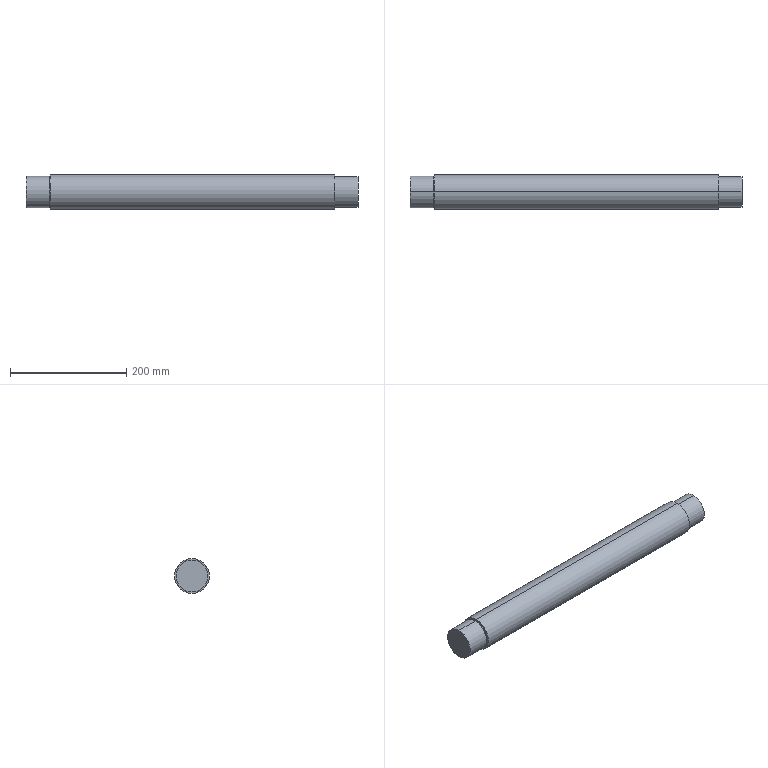Part | SolidWorks | features Revolution 1 | 1 solid | 13 faces | box 572 x 60 x 60 mm | volume 1573135 mm3 | cylinder 8 | plane 5 | commonest cylinder face diameters 53 x4 55 x2 60 x2
STEP:
#1=CARTESIAN_POINT('',(572.,0.,26.5));
#2=VERTEX_POINT('',#1);
#3=CARTESIAN_POINT('',(572.,0.,-26.5));
#4=VERTEX_POINT('',#3);
#5=CARTESIAN_POINT('',(572.,0.,0.));
#6=DIRECTION('',(-1.,0.,0.));
#7=DIRECTION('',(0.,0.,1.));
#8=AXIS2_PLACEMENT_3D('',#5,#6,#7);
#9=CIRCLE('',#8,26.5);
#10=EDGE_CURVE('',#2,#4,#9,.T.);
#11=ORIENTED_EDGE('',*,*,#10,.T.);
#12=CARTESIAN_POINT('',(532.,0.,-26.5));
#13=VERTEX_POINT('',#12);
#14=CARTESIAN_POINT('',(0.,0.,-26.5));
#15=DIRECTION('',(-1.,0.,0.));
#16=VECTOR('',#15,1000.);
#17=LINE('',#14,#16);
#18=EDGE_CURVE('',#4,#13,#17,.T.);
#19=ORIENTED_EDGE('',*,*,#18,.T.);
#20=CARTESIAN_POINT('',(532.,0.,26.5));
#21=VERTEX_POINT('',#20);
#22=CARTESIAN_POINT('',(532.,0.,0.));
#23=DIRECTION('',(-1.,0.,0.));
#24=DIRECTION('',(0.,0.,1.));
#25=AXIS2_PLACEMENT_3D('',#22,#23,#24);
#26=CIRCLE('',#25,26.5);
#27=EDGE_CURVE('',#21,#13,#26,.T.);
#28=ORIENTED_EDGE('',*,*,#27,.F.);
#29=CARTESIAN_POINT('',(0.,0.,26.5));
#30=DIRECTION('',(-1.,0.,0.));
#31=VECTOR('',#30,1000.);
#32=LINE('',#29,#31);
#33=EDGE_CURVE('',#2,#21,#32,.T.);
#34=ORIENTED_EDGE('',*,*,#33,.F.);
#35=EDGE_LOOP('',(#11,#19,#28,#34));
#36=FACE_OUTER_BOUND('',#35,.T.);
#37=CARTESIAN_POINT('',(0.,0.,0.));
#38=DIRECTION('',(-1.,0.,0.));
#39=DIRECTION('',(0.,0.,1.));
#40=AXIS2_PLACEMENT_3D('',#37,#38,#39);
#41=CYLINDRICAL_SURFACE('',#40,26.5);
#42=ADVANCED_FACE('',(#36),#41,.T.);
#43=CARTESIAN_POINT('',(532.,0.,30.));
#44=VERTEX_POINT('',#43);
#45=CARTESIAN_POINT('',(532.,0.,-30.));
#46=VERTEX_POINT('',#45);
#47=CARTESIAN_POINT('',(532.,0.,0.));
#48=DIRECTION('',(-1.,0.,0.));
#49=DIRECTION('',(0.,0.,1.));
#50=AXIS2_PLACEMENT_3D('',#47,#48,#49);
#51=CIRCLE('',#50,30.);
#52=EDGE_CURVE('',#44,#46,#51,.T.);
#53=ORIENTED_EDGE('',*,*,#52,.T.);
#54=CARTESIAN_POINT('',(42.,0.,-30.));
#55=VERTEX_POINT('',#54);
#56=CARTESIAN_POINT('',(0.,0.,-30.));
#57=DIRECTION('',(-1.,0.,0.));
#58=VECTOR('',#57,1000.);
#59=LINE('',#56,#58);
#60=EDGE_CURVE('',#46,#55,#59,.T.);
#61=ORIENTED_EDGE('',*,*,#60,.T.);
#62=CARTESIAN_POINT('',(42.,0.,30.));
#63=VERTEX_POINT('',#62);
#64=CARTESIAN_POINT('',(42.,0.,0.));
#65=DIRECTION('',(-1.,0.,0.));
#66=DIRECTION('',(0.,0.,1.));
#67=AXIS2_PLACEMENT_3D('',#64,#65,#66);
#68=CIRCLE('',#67,30.);
#69=EDGE_CURVE('',#63,#55,#68,.T.);
#70=ORIENTED_EDGE('',*,*,#69,.F.);
#71=CARTESIAN_POINT('',(0.,0.,30.));
#72=DIRECTION('',(-1.,0.,0.));
#73=VECTOR('',#72,1000.);
#74=LINE('',#71,#73);
#75=EDGE_CURVE('',#44,#63,#74,.T.);
#76=ORIENTED_EDGE('',*,*,#75,.F.);
#77=EDGE_LOOP('',(#53,#61,#70,#76));
#78=FACE_OUTER_BOUND('',#77,.T.);
#79=CARTESIAN_POINT('',(0.,0.,0.));
#80=DIRECTION('',(-1.,0.,0.));
#81=DIRECTION('',(0.,0.,1.));
#82=AXIS2_PLACEMENT_3D('',#79,#80,#81);
#83=CYLINDRICAL_SURFACE('',#82,30.);
#84=ADVANCED_FACE('',(#78),#83,.T.);
#85=CARTESIAN_POINT('',(42.,0.,26.5));
#86=VERTEX_POINT('',#85);
#87=CARTESIAN_POINT('',(42.,0.,-26.5));
#88=VERTEX_POINT('',#87);
#89=CARTESIAN_POINT('',(42.,0.,0.));
#90=DIRECTION('',(-1.,0.,0.));
#91=DIRECTION('',(0.,0.,1.));
#92=AXIS2_PLACEMENT_3D('',#89,#90,#91);
#93=CIRCLE('',#92,26.5);
#94=EDGE_CURVE('',#86,#88,#93,.T.);
#95=ORIENTED_EDGE('',*,*,#94,.T.);
#96=CARTESIAN_POINT('',(40.,0.,-26.5));
#97=VERTEX_POINT('',#96);
#98=CARTESIAN_POINT('',(0.,0.,-26.5));
#99=DIRECTION('',(-1.,0.,0.));
#100=VECTOR('',#99,1000.);
#101=LINE('',#98,#100);
#102=EDGE_CURVE('',#88,#97,#101,.T.);
#103=ORIENTED_EDGE('',*,*,#102,.T.);
#104=CARTESIAN_POINT('',(40.,0.,26.5));
#105=VERTEX_POINT('',#104);
#106=CARTESIAN_POINT('',(40.,0.,0.));
#107=DIRECTION('',(-1.,0.,0.));
#108=DIRECTION('',(0.,0.,1.));
#109=AXIS2_PLACEMENT_3D('',#106,#107,#108);
#110=CIRCLE('',#109,26.5);
#111=EDGE_CURVE('',#105,#97,#110,.T.);
#112=ORIENTED_EDGE('',*,*,#111,.F.);
#113=CARTESIAN_POINT('',(0.,0.,26.5));
#114=DIRECTION('',(-1.,0.,0.));
#115=VECTOR('',#114,1000.);
#116=LINE('',#113,#115);
#117=EDGE_CURVE('',#86,#105,#116,.T.);
#118=ORIENTED_EDGE('',*,*,#117,.F.);
#119=EDGE_LOOP('',(#95,#103,#112,#118));
#120=FACE_OUTER_BOUND('',#119,.T.);
#121=CARTESIAN_POINT('',(0.,0.,0.));
#122=DIRECTION('',(-1.,0.,0.));
#123=DIRECTION('',(0.,0.,1.));
#124=AXIS2_PLACEMENT_3D('',#121,#122,#123);
#125=CYLINDRICAL_SURFACE('',#124,26.5);
#126=ADVANCED_FACE('',(#120),#125,.T.);
#127=CARTESIAN_POINT('',(40.,0.,27.5));
#128=VERTEX_POINT('',#127);
#129=CARTESIAN_POINT('',(40.,0.,-27.5));
#130=VERTEX_POINT('',#129);
#131=CARTESIAN_POINT('',(40.,0.,0.));
#132=DIRECTION('',(-1.,0.,0.));
#133=DIRECTION('',(0.,0.,1.));
#134=AXIS2_PLACEMENT_3D('',#131,#132,#133);
#135=CIRCLE('',#134,27.5);
#136=EDGE_CURVE('',#128,#130,#135,.T.);
#137=ORIENTED_EDGE('',*,*,#136,.T.);
#138=CARTESIAN_POINT('',(0.,0.,-27.5));
#139=VERTEX_POINT('',#138);
#140=CARTESIAN_POINT('',(0.,0.,-27.5));
#141=DIRECTION('',(-1.,0.,0.));
#142=VECTOR('',#141,1000.);
#143=LINE('',#140,#142);
#144=EDGE_CURVE('',#130,#139,#143,.T.);
#145=ORIENTED_EDGE('',*,*,#144,.T.);
#146=CARTESIAN_POINT('',(0.,0.,27.5));
#147=VERTEX_POINT('',#146);
#148=CARTESIAN_POINT('',(0.,0.,0.));
#149=DIRECTION('',(-1.,0.,0.));
#150=DIRECTION('',(0.,0.,1.));
#151=AXIS2_PLACEMENT_3D('',#148,#149,#150);
#152=CIRCLE('',#151,27.5);
#153=EDGE_CURVE('',#147,#139,#152,.T.);
#154=ORIENTED_EDGE('',*,*,#153,.F.);
#155=CARTESIAN_POINT('',(0.,0.,27.5));
#156=DIRECTION('',(-1.,0.,0.));
#157=VECTOR('',#156,1000.);
#158=LINE('',#155,#157);
#159=EDGE_CURVE('',#128,#147,#158,.T.);
#160=ORIENTED_EDGE('',*,*,#159,.F.);
#161=EDGE_LOOP('',(#137,#145,#154,#160));
#162=FACE_OUTER_BOUND('',#161,.T.);
#163=CARTESIAN_POINT('',(0.,0.,0.));
#164=DIRECTION('',(-1.,0.,0.));
#165=DIRECTION('',(0.,0.,1.));
#166=AXIS2_PLACEMENT_3D('',#163,#164,#165);
#167=CYLINDRICAL_SURFACE('',#166,27.5);
#168=ADVANCED_FACE('',(#162),#167,.T.);
#169=ORIENTED_EDGE('',*,*,#153,.T.);
#170=CARTESIAN_POINT('',(0.,0.,0.));
#171=DIRECTION('',(-1.,0.,0.));
#172=DIRECTION('',(0.,0.,1.));
#173=AXIS2_PLACEMENT_3D('',#170,#171,#172);
#174=CIRCLE('',#173,27.5);
#175=EDGE_CURVE('',#139,#147,#174,.T.);
#176=ORIENTED_EDGE('',*,*,#175,.T.);
#177=EDGE_LOOP('',(#169,#176));
#178=FACE_OUTER_BOUND('',#177,.T.);
#179=CARTESIAN_POINT('',(0.,0.,0.));
#180=DIRECTION('',(1.,0.,0.));
#181=DIRECTION('',(0.,0.,-1.));
#182=AXIS2_PLACEMENT_3D('',#179,#180,#181);
#183=PLANE('',#182);
#184=ADVANCED_FACE('',(#178),#183,.F.);
#185=ORIENTED_EDGE('',*,*,#144,.F.);
#186=CARTESIAN_POINT('',(40.,0.,0.));
#187=DIRECTION('',(-1.,0.,0.));
#188=DIRECTION('',(0.,0.,1.));
#189=AXIS2_PLACEMENT_3D('',#186,#187,#188);
#190=CIRCLE('',#189,27.5);
#191=EDGE_CURVE('',#130,#128,#190,.T.);
#192=ORIENTED_EDGE('',*,*,#191,.T.);
#193=ORIENTED_EDGE('',*,*,#159,.T.);
#194=ORIENTED_EDGE('',*,*,#175,.F.);
#195=EDGE_LOOP('',(#185,#192,#193,#194));
#196=FACE_OUTER_BOUND('',#195,.T.);
#197=CARTESIAN_POINT('',(0.,0.,0.));
#198=DIRECTION('',(-1.,0.,0.));
#199=DIRECTION('',(0.,0.,1.));
#200=AXIS2_PLACEMENT_3D('',#197,#198,#199);
#201=CYLINDRICAL_SURFACE('',#200,27.5);
#202=ADVANCED_FACE('',(#196),#201,.T.);
#203=ORIENTED_EDGE('',*,*,#136,.F.);
#204=ORIENTED_EDGE('',*,*,#191,.F.);
#205=EDGE_LOOP('',(#203,#204));
#206=FACE_OUTER_BOUND('',#205,.T.);
#207=ORIENTED_EDGE('',*,*,#111,.T.);
#208=CARTESIAN_POINT('',(40.,0.,0.));
#209=DIRECTION('',(-1.,0.,0.));
#210=DIRECTION('',(0.,0.,1.));
#211=AXIS2_PLACEMENT_3D('',#208,#209,#210);
#212=CIRCLE('',#211,26.5);
#213=EDGE_CURVE('',#97,#105,#212,.T.);
#214=ORIENTED_EDGE('',*,*,#213,.T.);
#215=EDGE_LOOP('',(#207,#214));
#216=FACE_BOUND('',#215,.T.);
#217=CARTESIAN_POINT('',(40.,27.5,0.));
#218=DIRECTION('',(-1.,0.,0.));
#219=DIRECTION('',(0.,0.,1.));
#220=AXIS2_PLACEMENT_3D('',#217,#218,#219);
#221=PLANE('',#220);
#222=ADVANCED_FACE('',(#206,#216),#221,.F.);
#223=ORIENTED_EDGE('',*,*,#102,.F.);
#224=CARTESIAN_POINT('',(42.,0.,0.));
#225=DIRECTION('',(-1.,0.,0.));
#226=DIRECTION('',(0.,0.,1.));
#227=AXIS2_PLACEMENT_3D('',#224,#225,#226);
#228=CIRCLE('',#227,26.5);
#229=EDGE_CURVE('',#88,#86,#228,.T.);
#230=ORIENTED_EDGE('',*,*,#229,.T.);
#231=ORIENTED_EDGE('',*,*,#117,.T.);
#232=ORIENTED_EDGE('',*,*,#213,.F.);
#233=EDGE_LOOP('',(#223,#230,#231,#232));
#234=FACE_OUTER_BOUND('',#233,.T.);
#235=CARTESIAN_POINT('',(0.,0.,0.));
#236=DIRECTION('',(-1.,0.,0.));
#237=DIRECTION('',(0.,0.,1.));
#238=AXIS2_PLACEMENT_3D('',#235,#236,#237);
#239=CYLINDRICAL_SURFACE('',#238,26.5);
#240=ADVANCED_FACE('',(#234),#239,.T.);
#241=ORIENTED_EDGE('',*,*,#94,.F.);
#242=ORIENTED_EDGE('',*,*,#229,.F.);
#243=EDGE_LOOP('',(#241,#242));
#244=FACE_BOUND('',#243,.T.);
#245=ORIENTED_EDGE('',*,*,#69,.T.);
#246=CARTESIAN_POINT('',(42.,0.,0.));
#247=DIRECTION('',(-1.,0.,0.));
#248=DIRECTION('',(0.,0.,1.));
#249=AXIS2_PLACEMENT_3D('',#246,#247,#248);
#250=CIRCLE('',#249,30.);
#251=EDGE_CURVE('',#55,#63,#250,.T.);
#252=ORIENTED_EDGE('',*,*,#251,.T.);
#253=EDGE_LOOP('',(#245,#252));
#254=FACE_OUTER_BOUND('',#253,.T.);
#255=CARTESIAN_POINT('',(42.,26.5,0.));
#256=DIRECTION('',(1.,0.,0.));
#257=DIRECTION('',(0.,0.,-1.));
#258=AXIS2_PLACEMENT_3D('',#255,#256,#257);
#259=PLANE('',#258);
#260=ADVANCED_FACE('',(#244,#254),#259,.F.);
#261=ORIENTED_EDGE('',*,*,#60,.F.);
#262=CARTESIAN_POINT('',(532.,0.,0.));
#263=DIRECTION('',(-1.,0.,0.));
#264=DIRECTION('',(0.,0.,1.));
#265=AXIS2_PLACEMENT_3D('',#262,#263,#264);
#266=CIRCLE('',#265,30.);
#267=EDGE_CURVE('',#46,#44,#266,.T.);
#268=ORIENTED_EDGE('',*,*,#267,.T.);
#269=ORIENTED_EDGE('',*,*,#75,.T.);
#270=ORIENTED_EDGE('',*,*,#251,.F.);
#271=EDGE_LOOP('',(#261,#268,#269,#270));
#272=FACE_OUTER_BOUND('',#271,.T.);
#273=CARTESIAN_POINT('',(0.,0.,0.));
#274=DIRECTION('',(-1.,0.,0.));
#275=DIRECTION('',(0.,0.,1.));
#276=AXIS2_PLACEMENT_3D('',#273,#274,#275);
#277=CYLINDRICAL_SURFACE('',#276,30.);
#278=ADVANCED_FACE('',(#272),#277,.T.);
#279=ORIENTED_EDGE('',*,*,#52,.F.);
#280=ORIENTED_EDGE('',*,*,#267,.F.);
#281=EDGE_LOOP('',(#279,#280));
#282=FACE_OUTER_BOUND('',#281,.T.);
#283=ORIENTED_EDGE('',*,*,#27,.T.);
#284=CARTESIAN_POINT('',(532.,0.,0.));
#285=DIRECTION('',(-1.,0.,0.));
#286=DIRECTION('',(0.,0.,1.));
#287=AXIS2_PLACEMENT_3D('',#284,#285,#286);
#288=CIRCLE('',#287,26.5);
#289=EDGE_CURVE('',#13,#21,#288,.T.);
#290=ORIENTED_EDGE('',*,*,#289,.T.);
#291=EDGE_LOOP('',(#283,#290));
#292=FACE_BOUND('',#291,.T.);
#293=CARTESIAN_POINT('',(532.,30.,0.));
#294=DIRECTION('',(-1.,0.,0.));
#295=DIRECTION('',(0.,0.,1.));
#296=AXIS2_PLACEMENT_3D('',#293,#294,#295);
#297=PLANE('',#296);
#298=ADVANCED_FACE('',(#282,#292),#297,.F.);
#299=ORIENTED_EDGE('',*,*,#18,.F.);
#300=CARTESIAN_POINT('',(572.,0.,0.));
#301=DIRECTION('',(-1.,0.,0.));
#302=DIRECTION('',(0.,0.,1.));
#303=AXIS2_PLACEMENT_3D('',#300,#301,#302);
#304=CIRCLE('',#303,26.5);
#305=EDGE_CURVE('',#4,#2,#304,.T.);
#306=ORIENTED_EDGE('',*,*,#305,.T.);
#307=ORIENTED_EDGE('',*,*,#33,.T.);
#308=ORIENTED_EDGE('',*,*,#289,.F.);
#309=EDGE_LOOP('',(#299,#306,#307,#308));
#310=FACE_OUTER_BOUND('',#309,.T.);
#311=CARTESIAN_POINT('',(0.,0.,0.));
#312=DIRECTION('',(-1.,0.,0.));
#313=DIRECTION('',(0.,0.,1.));
#314=AXIS2_PLACEMENT_3D('',#311,#312,#313);
#315=CYLINDRICAL_SURFACE('',#314,26.5);
#316=ADVANCED_FACE('',(#310),#315,.T.);
#317=ORIENTED_EDGE('',*,*,#10,.F.);
#318=ORIENTED_EDGE('',*,*,#305,.F.);
#319=EDGE_LOOP('',(#317,#318));
#320=FACE_OUTER_BOUND('',#319,.T.);
#321=CARTESIAN_POINT('',(572.,26.5,0.));
#322=DIRECTION('',(-1.,0.,0.));
#323=DIRECTION('',(0.,0.,1.));
#324=AXIS2_PLACEMENT_3D('',#321,#322,#323);
#325=PLANE('',#324);
#326=ADVANCED_FACE('',(#320),#325,.F.);
#327=CLOSED_SHELL('',(#42,#84,#126,#168,#184,#202,#222,#240,#260,#278,#298,#316,#326));
#328=MANIFOLD_SOLID_BREP('',#327);
#329=CARTESIAN_POINT('',(0.,0.,0.));
#330=DIRECTION('',(0.,0.,1.));
#331=DIRECTION('',(1.,0.,0.));
#332=AXIS2_PLACEMENT_3D('',#329,#330,#331);
#333=(LENGTH_UNIT()NAMED_UNIT(*)SI_UNIT(.MILLI.,.METRE.));
#334=UNCERTAINTY_MEASURE_WITH_UNIT(LENGTH_MEASURE(0.00001),#333,'','');
#335=(NAMED_UNIT(*)PLANE_ANGLE_UNIT()SI_UNIT($,.RADIAN.));
#336=(NAMED_UNIT(*)SI_UNIT($,.STERADIAN.)SOLID_ANGLE_UNIT());
#337=(GEOMETRIC_REPRESENTATION_CONTEXT(3)GLOBAL_UNCERTAINTY_ASSIGNED_CONTEXT((#334))GLOBAL_UNIT_ASSIGNED_CONTEXT((#333,#335,#336))REPRESENTATION_CONTEXT('',''));
#338=ADVANCED_BREP_SHAPE_REPRESENTATION('',(#328,#332),#337);